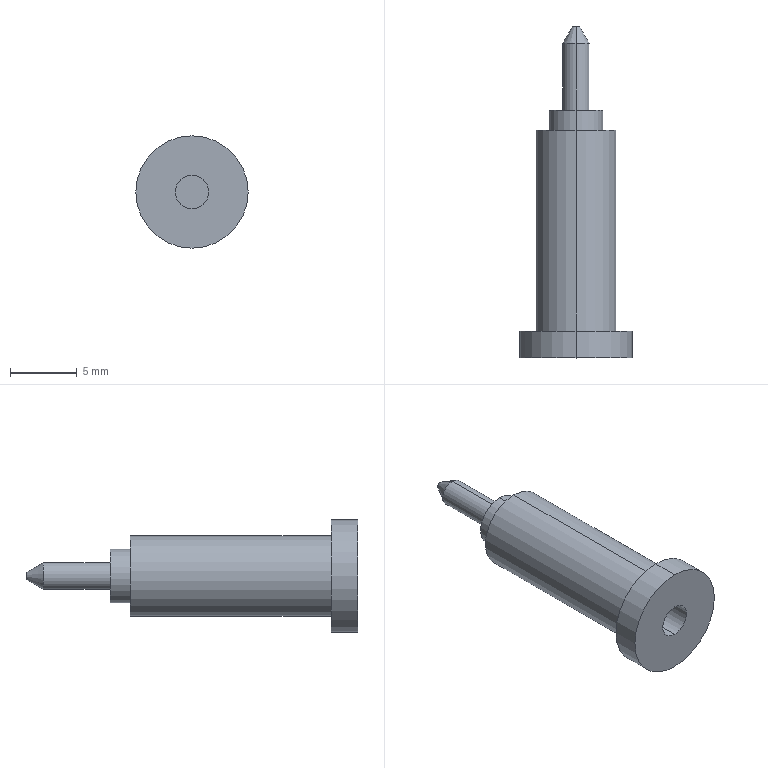Part | SolidWorks | features Revolution 1 | 1 solid | 18 faces | box 8.4 x 24.799 x 8.4 mm | volume 541.841 mm3 | cylinder 10 | plane 6 | cone 2 | commonest cylinder face diameters 2 x2 2.5 x2 4 x2 6 x2 8.4 x2
STEP:
#1=CARTESIAN_POINT('',(0.,6.,1.25));
#2=VERTEX_POINT('',#1);
#3=CARTESIAN_POINT('',(0.,6.,-1.25));
#4=VERTEX_POINT('',#3);
#5=CARTESIAN_POINT('',(0.,6.,0.));
#6=DIRECTION('',(0.,-1.,0.));
#7=DIRECTION('',(0.,0.,-1.));
#8=AXIS2_PLACEMENT_3D('',#5,#6,#7);
#9=CIRCLE('',#8,1.25);
#10=EDGE_CURVE('',#2,#4,#9,.T.);
#11=ORIENTED_EDGE('',*,*,#10,.F.);
#12=CARTESIAN_POINT('',(0.,0.,1.25));
#13=VERTEX_POINT('',#12);
#14=CARTESIAN_POINT('',(0.,0.,1.25));
#15=DIRECTION('',(0.,-1.,0.));
#16=VECTOR('',#15,1000.);
#17=LINE('',#14,#16);
#18=EDGE_CURVE('',#2,#13,#17,.T.);
#19=ORIENTED_EDGE('',*,*,#18,.T.);
#20=CARTESIAN_POINT('',(0.,0.,-1.25));
#21=VERTEX_POINT('',#20);
#22=CARTESIAN_POINT('',(0.,0.,0.));
#23=DIRECTION('',(0.,-1.,0.));
#24=DIRECTION('',(0.,0.,-1.));
#25=AXIS2_PLACEMENT_3D('',#22,#23,#24);
#26=CIRCLE('',#25,1.25);
#27=EDGE_CURVE('',#13,#21,#26,.T.);
#28=ORIENTED_EDGE('',*,*,#27,.T.);
#29=CARTESIAN_POINT('',(0.,0.,-1.25));
#30=DIRECTION('',(0.,-1.,0.));
#31=VECTOR('',#30,1000.);
#32=LINE('',#29,#31);
#33=EDGE_CURVE('',#4,#21,#32,.T.);
#34=ORIENTED_EDGE('',*,*,#33,.F.);
#35=EDGE_LOOP('',(#11,#19,#28,#34));
#36=FACE_OUTER_BOUND('',#35,.T.);
#37=CARTESIAN_POINT('',(0.,0.,0.));
#38=DIRECTION('',(0.,-1.,0.));
#39=DIRECTION('',(0.,0.,-1.));
#40=AXIS2_PLACEMENT_3D('',#37,#38,#39);
#41=CYLINDRICAL_SURFACE('',#40,1.25);
#42=ADVANCED_FACE('',(#36),#41,.F.);
#43=CARTESIAN_POINT('',(0.,24.799,-0.25));
#44=VERTEX_POINT('',#43);
#45=CARTESIAN_POINT('',(0.,24.799,0.25));
#46=VERTEX_POINT('',#45);
#47=CARTESIAN_POINT('',(0.,24.799,0.));
#48=DIRECTION('',(0.,-1.,0.));
#49=DIRECTION('',(0.,0.,-1.));
#50=AXIS2_PLACEMENT_3D('',#47,#48,#49);
#51=CIRCLE('',#50,0.25);
#52=EDGE_CURVE('',#44,#46,#51,.T.);
#53=ORIENTED_EDGE('',*,*,#52,.T.);
#54=CARTESIAN_POINT('',(0.,23.5,1.));
#55=VERTEX_POINT('',#54);
#56=CARTESIAN_POINT('',(0.,24.799,0.25));
#57=DIRECTION('',(0.,-0.866,0.5));
#58=VECTOR('',#57,1000.);
#59=LINE('',#56,#58);
#60=EDGE_CURVE('',#46,#55,#59,.T.);
#61=ORIENTED_EDGE('',*,*,#60,.T.);
#62=CARTESIAN_POINT('',(0.,23.5,-1.));
#63=VERTEX_POINT('',#62);
#64=CARTESIAN_POINT('',(0.,23.5,0.));
#65=DIRECTION('',(0.,-1.,0.));
#66=DIRECTION('',(0.,0.,-1.));
#67=AXIS2_PLACEMENT_3D('',#64,#65,#66);
#68=CIRCLE('',#67,1.);
#69=EDGE_CURVE('',#63,#55,#68,.T.);
#70=ORIENTED_EDGE('',*,*,#69,.F.);
#71=CARTESIAN_POINT('',(0.,24.799,-0.25));
#72=DIRECTION('',(0.,-0.866,-0.5));
#73=VECTOR('',#72,1000.);
#74=LINE('',#71,#73);
#75=EDGE_CURVE('',#44,#63,#74,.T.);
#76=ORIENTED_EDGE('',*,*,#75,.F.);
#77=EDGE_LOOP('',(#53,#61,#70,#76));
#78=FACE_OUTER_BOUND('',#77,.T.);
#79=CARTESIAN_POINT('',(0.,24.799,0.));
#80=DIRECTION('',(0.,-1.,0.));
#81=DIRECTION('',(0.,0.,-1.));
#82=AXIS2_PLACEMENT_3D('',#79,#80,#81);
#83=CONICAL_SURFACE('',#82,0.25,0.5236);
#84=ADVANCED_FACE('',(#78),#83,.T.);
#85=ORIENTED_EDGE('',*,*,#69,.T.);
#86=CARTESIAN_POINT('',(0.,18.5,1.));
#87=VERTEX_POINT('',#86);
#88=CARTESIAN_POINT('',(0.,0.,1.));
#89=DIRECTION('',(0.,-1.,0.));
#90=VECTOR('',#89,1000.);
#91=LINE('',#88,#90);
#92=EDGE_CURVE('',#55,#87,#91,.T.);
#93=ORIENTED_EDGE('',*,*,#92,.T.);
#94=CARTESIAN_POINT('',(0.,18.5,-1.));
#95=VERTEX_POINT('',#94);
#96=CARTESIAN_POINT('',(0.,18.5,0.));
#97=DIRECTION('',(0.,-1.,0.));
#98=DIRECTION('',(0.,0.,-1.));
#99=AXIS2_PLACEMENT_3D('',#96,#97,#98);
#100=CIRCLE('',#99,1.);
#101=EDGE_CURVE('',#95,#87,#100,.T.);
#102=ORIENTED_EDGE('',*,*,#101,.F.);
#103=CARTESIAN_POINT('',(0.,0.,-1.));
#104=DIRECTION('',(0.,-1.,0.));
#105=VECTOR('',#104,1000.);
#106=LINE('',#103,#105);
#107=EDGE_CURVE('',#63,#95,#106,.T.);
#108=ORIENTED_EDGE('',*,*,#107,.F.);
#109=EDGE_LOOP('',(#85,#93,#102,#108));
#110=FACE_OUTER_BOUND('',#109,.T.);
#111=CARTESIAN_POINT('',(0.,0.,0.));
#112=DIRECTION('',(0.,-1.,0.));
#113=DIRECTION('',(0.,0.,-1.));
#114=AXIS2_PLACEMENT_3D('',#111,#112,#113);
#115=CYLINDRICAL_SURFACE('',#114,1.);
#116=ADVANCED_FACE('',(#110),#115,.T.);
#117=CARTESIAN_POINT('',(0.,18.5,-2.));
#118=VERTEX_POINT('',#117);
#119=CARTESIAN_POINT('',(0.,18.5,2.));
#120=VERTEX_POINT('',#119);
#121=CARTESIAN_POINT('',(0.,18.5,0.));
#122=DIRECTION('',(0.,-1.,0.));
#123=DIRECTION('',(0.,0.,-1.));
#124=AXIS2_PLACEMENT_3D('',#121,#122,#123);
#125=CIRCLE('',#124,2.);
#126=EDGE_CURVE('',#118,#120,#125,.T.);
#127=ORIENTED_EDGE('',*,*,#126,.T.);
#128=CARTESIAN_POINT('',(0.,17.,2.));
#129=VERTEX_POINT('',#128);
#130=CARTESIAN_POINT('',(0.,0.,2.));
#131=DIRECTION('',(0.,-1.,0.));
#132=VECTOR('',#131,1000.);
#133=LINE('',#130,#132);
#134=EDGE_CURVE('',#120,#129,#133,.T.);
#135=ORIENTED_EDGE('',*,*,#134,.T.);
#136=CARTESIAN_POINT('',(0.,17.,-2.));
#137=VERTEX_POINT('',#136);
#138=CARTESIAN_POINT('',(0.,17.,0.));
#139=DIRECTION('',(0.,-1.,0.));
#140=DIRECTION('',(0.,0.,-1.));
#141=AXIS2_PLACEMENT_3D('',#138,#139,#140);
#142=CIRCLE('',#141,2.);
#143=EDGE_CURVE('',#137,#129,#142,.T.);
#144=ORIENTED_EDGE('',*,*,#143,.F.);
#145=CARTESIAN_POINT('',(0.,0.,-2.));
#146=DIRECTION('',(0.,-1.,0.));
#147=VECTOR('',#146,1000.);
#148=LINE('',#145,#147);
#149=EDGE_CURVE('',#118,#137,#148,.T.);
#150=ORIENTED_EDGE('',*,*,#149,.F.);
#151=EDGE_LOOP('',(#127,#135,#144,#150));
#152=FACE_OUTER_BOUND('',#151,.T.);
#153=CARTESIAN_POINT('',(0.,0.,0.));
#154=DIRECTION('',(0.,-1.,0.));
#155=DIRECTION('',(0.,0.,-1.));
#156=AXIS2_PLACEMENT_3D('',#153,#154,#155);
#157=CYLINDRICAL_SURFACE('',#156,2.);
#158=ADVANCED_FACE('',(#152),#157,.T.);
#159=CARTESIAN_POINT('',(0.,17.,-3.));
#160=VERTEX_POINT('',#159);
#161=CARTESIAN_POINT('',(0.,17.,3.));
#162=VERTEX_POINT('',#161);
#163=CARTESIAN_POINT('',(0.,17.,0.));
#164=DIRECTION('',(0.,-1.,0.));
#165=DIRECTION('',(0.,0.,-1.));
#166=AXIS2_PLACEMENT_3D('',#163,#164,#165);
#167=CIRCLE('',#166,3.);
#168=EDGE_CURVE('',#160,#162,#167,.T.);
#169=ORIENTED_EDGE('',*,*,#168,.T.);
#170=CARTESIAN_POINT('',(0.,2.,3.));
#171=VERTEX_POINT('',#170);
#172=CARTESIAN_POINT('',(0.,0.,3.));
#173=DIRECTION('',(0.,-1.,0.));
#174=VECTOR('',#173,1000.);
#175=LINE('',#172,#174);
#176=EDGE_CURVE('',#162,#171,#175,.T.);
#177=ORIENTED_EDGE('',*,*,#176,.T.);
#178=CARTESIAN_POINT('',(0.,2.,-3.));
#179=VERTEX_POINT('',#178);
#180=CARTESIAN_POINT('',(0.,2.,0.));
#181=DIRECTION('',(0.,-1.,0.));
#182=DIRECTION('',(0.,0.,-1.));
#183=AXIS2_PLACEMENT_3D('',#180,#181,#182);
#184=CIRCLE('',#183,3.);
#185=EDGE_CURVE('',#179,#171,#184,.T.);
#186=ORIENTED_EDGE('',*,*,#185,.F.);
#187=CARTESIAN_POINT('',(0.,0.,-3.));
#188=DIRECTION('',(0.,-1.,0.));
#189=VECTOR('',#188,1000.);
#190=LINE('',#187,#189);
#191=EDGE_CURVE('',#160,#179,#190,.T.);
#192=ORIENTED_EDGE('',*,*,#191,.F.);
#193=EDGE_LOOP('',(#169,#177,#186,#192));
#194=FACE_OUTER_BOUND('',#193,.T.);
#195=CARTESIAN_POINT('',(0.,0.,0.));
#196=DIRECTION('',(0.,-1.,0.));
#197=DIRECTION('',(0.,0.,-1.));
#198=AXIS2_PLACEMENT_3D('',#195,#196,#197);
#199=CYLINDRICAL_SURFACE('',#198,3.);
#200=ADVANCED_FACE('',(#194),#199,.T.);
#201=CARTESIAN_POINT('',(0.,2.,-4.2));
#202=VERTEX_POINT('',#201);
#203=CARTESIAN_POINT('',(0.,2.,4.2));
#204=VERTEX_POINT('',#203);
#205=CARTESIAN_POINT('',(0.,2.,0.));
#206=DIRECTION('',(0.,-1.,0.));
#207=DIRECTION('',(0.,0.,-1.));
#208=AXIS2_PLACEMENT_3D('',#205,#206,#207);
#209=CIRCLE('',#208,4.2);
#210=EDGE_CURVE('',#202,#204,#209,.T.);
#211=ORIENTED_EDGE('',*,*,#210,.T.);
#212=CARTESIAN_POINT('',(0.,0.,4.2));
#213=VERTEX_POINT('',#212);
#214=CARTESIAN_POINT('',(0.,0.,4.2));
#215=DIRECTION('',(0.,-1.,0.));
#216=VECTOR('',#215,1000.);
#217=LINE('',#214,#216);
#218=EDGE_CURVE('',#204,#213,#217,.T.);
#219=ORIENTED_EDGE('',*,*,#218,.T.);
#220=CARTESIAN_POINT('',(0.,0.,-4.2));
#221=VERTEX_POINT('',#220);
#222=CARTESIAN_POINT('',(0.,0.,0.));
#223=DIRECTION('',(0.,-1.,0.));
#224=DIRECTION('',(0.,0.,-1.));
#225=AXIS2_PLACEMENT_3D('',#222,#223,#224);
#226=CIRCLE('',#225,4.2);
#227=EDGE_CURVE('',#221,#213,#226,.T.);
#228=ORIENTED_EDGE('',*,*,#227,.F.);
#229=CARTESIAN_POINT('',(0.,0.,-4.2));
#230=DIRECTION('',(0.,-1.,0.));
#231=VECTOR('',#230,1000.);
#232=LINE('',#229,#231);
#233=EDGE_CURVE('',#202,#221,#232,.T.);
#234=ORIENTED_EDGE('',*,*,#233,.F.);
#235=EDGE_LOOP('',(#211,#219,#228,#234));
#236=FACE_OUTER_BOUND('',#235,.T.);
#237=CARTESIAN_POINT('',(0.,0.,0.));
#238=DIRECTION('',(0.,-1.,0.));
#239=DIRECTION('',(0.,0.,-1.));
#240=AXIS2_PLACEMENT_3D('',#237,#238,#239);
#241=CYLINDRICAL_SURFACE('',#240,4.2);
#242=ADVANCED_FACE('',(#236),#241,.T.);
#243=ORIENTED_EDGE('',*,*,#218,.F.);
#244=CARTESIAN_POINT('',(0.,2.,0.));
#245=DIRECTION('',(0.,-1.,0.));
#246=DIRECTION('',(0.,0.,-1.));
#247=AXIS2_PLACEMENT_3D('',#244,#245,#246);
#248=CIRCLE('',#247,4.2);
#249=EDGE_CURVE('',#204,#202,#248,.T.);
#250=ORIENTED_EDGE('',*,*,#249,.T.);
#251=ORIENTED_EDGE('',*,*,#233,.T.);
#252=CARTESIAN_POINT('',(0.,0.,0.));
#253=DIRECTION('',(0.,-1.,0.));
#254=DIRECTION('',(0.,0.,-1.));
#255=AXIS2_PLACEMENT_3D('',#252,#253,#254);
#256=CIRCLE('',#255,4.2);
#257=EDGE_CURVE('',#213,#221,#256,.T.);
#258=ORIENTED_EDGE('',*,*,#257,.F.);
#259=EDGE_LOOP('',(#243,#250,#251,#258));
#260=FACE_OUTER_BOUND('',#259,.T.);
#261=CARTESIAN_POINT('',(0.,0.,0.));
#262=DIRECTION('',(0.,-1.,0.));
#263=DIRECTION('',(0.,0.,-1.));
#264=AXIS2_PLACEMENT_3D('',#261,#262,#263);
#265=CYLINDRICAL_SURFACE('',#264,4.2);
#266=ADVANCED_FACE('',(#260),#265,.T.);
#267=ORIENTED_EDGE('',*,*,#210,.F.);
#268=ORIENTED_EDGE('',*,*,#249,.F.);
#269=EDGE_LOOP('',(#267,#268));
#270=FACE_OUTER_BOUND('',#269,.T.);
#271=ORIENTED_EDGE('',*,*,#185,.T.);
#272=CARTESIAN_POINT('',(0.,2.,0.));
#273=DIRECTION('',(0.,-1.,0.));
#274=DIRECTION('',(0.,0.,-1.));
#275=AXIS2_PLACEMENT_3D('',#272,#273,#274);
#276=CIRCLE('',#275,3.);
#277=EDGE_CURVE('',#171,#179,#276,.T.);
#278=ORIENTED_EDGE('',*,*,#277,.T.);
#279=EDGE_LOOP('',(#271,#278));
#280=FACE_BOUND('',#279,.T.);
#281=CARTESIAN_POINT('',(-4.2,2.,0.));
#282=DIRECTION('',(0.,-1.,0.));
#283=DIRECTION('',(0.,0.,-1.));
#284=AXIS2_PLACEMENT_3D('',#281,#282,#283);
#285=PLANE('',#284);
#286=ADVANCED_FACE('',(#270,#280),#285,.F.);
#287=ORIENTED_EDGE('',*,*,#176,.F.);
#288=CARTESIAN_POINT('',(0.,17.,0.));
#289=DIRECTION('',(0.,-1.,0.));
#290=DIRECTION('',(0.,0.,-1.));
#291=AXIS2_PLACEMENT_3D('',#288,#289,#290);
#292=CIRCLE('',#291,3.);
#293=EDGE_CURVE('',#162,#160,#292,.T.);
#294=ORIENTED_EDGE('',*,*,#293,.T.);
#295=ORIENTED_EDGE('',*,*,#191,.T.);
#296=ORIENTED_EDGE('',*,*,#277,.F.);
#297=EDGE_LOOP('',(#287,#294,#295,#296));
#298=FACE_OUTER_BOUND('',#297,.T.);
#299=CARTESIAN_POINT('',(0.,0.,0.));
#300=DIRECTION('',(0.,-1.,0.));
#301=DIRECTION('',(0.,0.,-1.));
#302=AXIS2_PLACEMENT_3D('',#299,#300,#301);
#303=CYLINDRICAL_SURFACE('',#302,3.);
#304=ADVANCED_FACE('',(#298),#303,.T.);
#305=ORIENTED_EDGE('',*,*,#168,.F.);
#306=ORIENTED_EDGE('',*,*,#293,.F.);
#307=EDGE_LOOP('',(#305,#306));
#308=FACE_OUTER_BOUND('',#307,.T.);
#309=ORIENTED_EDGE('',*,*,#143,.T.);
#310=CARTESIAN_POINT('',(0.,17.,0.));
#311=DIRECTION('',(0.,-1.,0.));
#312=DIRECTION('',(0.,0.,-1.));
#313=AXIS2_PLACEMENT_3D('',#310,#311,#312);
#314=CIRCLE('',#313,2.);
#315=EDGE_CURVE('',#129,#137,#314,.T.);
#316=ORIENTED_EDGE('',*,*,#315,.T.);
#317=EDGE_LOOP('',(#309,#316));
#318=FACE_BOUND('',#317,.T.);
#319=CARTESIAN_POINT('',(-3.,17.,0.));
#320=DIRECTION('',(0.,-1.,0.));
#321=DIRECTION('',(0.,0.,-1.));
#322=AXIS2_PLACEMENT_3D('',#319,#320,#321);
#323=PLANE('',#322);
#324=ADVANCED_FACE('',(#308,#318),#323,.F.);
#325=ORIENTED_EDGE('',*,*,#134,.F.);
#326=CARTESIAN_POINT('',(0.,18.5,0.));
#327=DIRECTION('',(0.,-1.,0.));
#328=DIRECTION('',(0.,0.,-1.));
#329=AXIS2_PLACEMENT_3D('',#326,#327,#328);
#330=CIRCLE('',#329,2.);
#331=EDGE_CURVE('',#120,#118,#330,.T.);
#332=ORIENTED_EDGE('',*,*,#331,.T.);
#333=ORIENTED_EDGE('',*,*,#149,.T.);
#334=ORIENTED_EDGE('',*,*,#315,.F.);
#335=EDGE_LOOP('',(#325,#332,#333,#334));
#336=FACE_OUTER_BOUND('',#335,.T.);
#337=CARTESIAN_POINT('',(0.,0.,0.));
#338=DIRECTION('',(0.,-1.,0.));
#339=DIRECTION('',(0.,0.,-1.));
#340=AXIS2_PLACEMENT_3D('',#337,#338,#339);
#341=CYLINDRICAL_SURFACE('',#340,2.);
#342=ADVANCED_FACE('',(#336),#341,.T.);
#343=ORIENTED_EDGE('',*,*,#126,.F.);
#344=ORIENTED_EDGE('',*,*,#331,.F.);
#345=EDGE_LOOP('',(#343,#344));
#346=FACE_OUTER_BOUND('',#345,.T.);
#347=ORIENTED_EDGE('',*,*,#101,.T.);
#348=CARTESIAN_POINT('',(0.,18.5,0.));
#349=DIRECTION('',(0.,-1.,0.));
#350=DIRECTION('',(0.,0.,-1.));
#351=AXIS2_PLACEMENT_3D('',#348,#349,#350);
#352=CIRCLE('',#351,1.);
#353=EDGE_CURVE('',#87,#95,#352,.T.);
#354=ORIENTED_EDGE('',*,*,#353,.T.);
#355=EDGE_LOOP('',(#347,#354));
#356=FACE_BOUND('',#355,.T.);
#357=CARTESIAN_POINT('',(-2.,18.5,0.));
#358=DIRECTION('',(0.,-1.,0.));
#359=DIRECTION('',(0.,0.,-1.));
#360=AXIS2_PLACEMENT_3D('',#357,#358,#359);
#361=PLANE('',#360);
#362=ADVANCED_FACE('',(#346,#356),#361,.F.);
#363=ORIENTED_EDGE('',*,*,#92,.F.);
#364=CARTESIAN_POINT('',(0.,23.5,0.));
#365=DIRECTION('',(0.,-1.,0.));
#366=DIRECTION('',(0.,0.,-1.));
#367=AXIS2_PLACEMENT_3D('',#364,#365,#366);
#368=CIRCLE('',#367,1.);
#369=EDGE_CURVE('',#55,#63,#368,.T.);
#370=ORIENTED_EDGE('',*,*,#369,.T.);
#371=ORIENTED_EDGE('',*,*,#107,.T.);
#372=ORIENTED_EDGE('',*,*,#353,.F.);
#373=EDGE_LOOP('',(#363,#370,#371,#372));
#374=FACE_OUTER_BOUND('',#373,.T.);
#375=CARTESIAN_POINT('',(0.,0.,0.));
#376=DIRECTION('',(0.,-1.,0.));
#377=DIRECTION('',(0.,0.,-1.));
#378=AXIS2_PLACEMENT_3D('',#375,#376,#377);
#379=CYLINDRICAL_SURFACE('',#378,1.);
#380=ADVANCED_FACE('',(#374),#379,.T.);
#381=ORIENTED_EDGE('',*,*,#60,.F.);
#382=CARTESIAN_POINT('',(0.,24.799,0.));
#383=DIRECTION('',(0.,-1.,0.));
#384=DIRECTION('',(0.,0.,-1.));
#385=AXIS2_PLACEMENT_3D('',#382,#383,#384);
#386=CIRCLE('',#385,0.25);
#387=EDGE_CURVE('',#46,#44,#386,.T.);
#388=ORIENTED_EDGE('',*,*,#387,.T.);
#389=ORIENTED_EDGE('',*,*,#75,.T.);
#390=ORIENTED_EDGE('',*,*,#369,.F.);
#391=EDGE_LOOP('',(#381,#388,#389,#390));
#392=FACE_OUTER_BOUND('',#391,.T.);
#393=CARTESIAN_POINT('',(0.,24.799,0.));
#394=DIRECTION('',(0.,-1.,0.));
#395=DIRECTION('',(0.,0.,-1.));
#396=AXIS2_PLACEMENT_3D('',#393,#394,#395);
#397=CONICAL_SURFACE('',#396,0.25,0.5236);
#398=ADVANCED_FACE('',(#392),#397,.T.);
#399=ORIENTED_EDGE('',*,*,#52,.F.);
#400=ORIENTED_EDGE('',*,*,#387,.F.);
#401=EDGE_LOOP('',(#399,#400));
#402=FACE_OUTER_BOUND('',#401,.T.);
#403=CARTESIAN_POINT('',(-0.25,24.799,0.));
#404=DIRECTION('',(0.,-1.,0.));
#405=DIRECTION('',(0.,0.,-1.));
#406=AXIS2_PLACEMENT_3D('',#403,#404,#405);
#407=PLANE('',#406);
#408=ADVANCED_FACE('',(#402),#407,.F.);
#409=CARTESIAN_POINT('',(0.,6.,0.));
#410=DIRECTION('',(0.,-1.,0.));
#411=DIRECTION('',(0.,0.,-1.));
#412=AXIS2_PLACEMENT_3D('',#409,#410,#411);
#413=CIRCLE('',#412,1.25);
#414=EDGE_CURVE('',#4,#2,#413,.T.);
#415=ORIENTED_EDGE('',*,*,#414,.T.);
#416=ORIENTED_EDGE('',*,*,#10,.T.);
#417=EDGE_LOOP('',(#415,#416));
#418=FACE_OUTER_BOUND('',#417,.T.);
#419=CARTESIAN_POINT('',(-1.25,6.,0.));
#420=DIRECTION('',(0.,1.,0.));
#421=DIRECTION('',(0.,0.,1.));
#422=AXIS2_PLACEMENT_3D('',#419,#420,#421);
#423=PLANE('',#422);
#424=ADVANCED_FACE('',(#418),#423,.F.);
#425=ORIENTED_EDGE('',*,*,#18,.F.);
#426=ORIENTED_EDGE('',*,*,#414,.F.);
#427=ORIENTED_EDGE('',*,*,#33,.T.);
#428=CARTESIAN_POINT('',(0.,0.,0.));
#429=DIRECTION('',(0.,-1.,0.));
#430=DIRECTION('',(0.,0.,-1.));
#431=AXIS2_PLACEMENT_3D('',#428,#429,#430);
#432=CIRCLE('',#431,1.25);
#433=EDGE_CURVE('',#21,#13,#432,.T.);
#434=ORIENTED_EDGE('',*,*,#433,.T.);
#435=EDGE_LOOP('',(#425,#426,#427,#434));
#436=FACE_OUTER_BOUND('',#435,.T.);
#437=CARTESIAN_POINT('',(0.,0.,0.));
#438=DIRECTION('',(0.,-1.,0.));
#439=DIRECTION('',(0.,0.,-1.));
#440=AXIS2_PLACEMENT_3D('',#437,#438,#439);
#441=CYLINDRICAL_SURFACE('',#440,1.25);
#442=ADVANCED_FACE('',(#436),#441,.F.);
#443=ORIENTED_EDGE('',*,*,#433,.F.);
#444=ORIENTED_EDGE('',*,*,#27,.F.);
#445=EDGE_LOOP('',(#443,#444));
#446=FACE_BOUND('',#445,.T.);
#447=ORIENTED_EDGE('',*,*,#227,.T.);
#448=ORIENTED_EDGE('',*,*,#257,.T.);
#449=EDGE_LOOP('',(#447,#448));
#450=FACE_OUTER_BOUND('',#449,.T.);
#451=CARTESIAN_POINT('',(-1.25,0.,0.));
#452=DIRECTION('',(0.,1.,0.));
#453=DIRECTION('',(0.,0.,1.));
#454=AXIS2_PLACEMENT_3D('',#451,#452,#453);
#455=PLANE('',#454);
#456=ADVANCED_FACE('',(#446,#450),#455,.F.);
#457=CLOSED_SHELL('',(#42,#84,#116,#158,#200,#242,#266,#286,#304,#324,#342,#362,#380,#398,#408,#424,#442,#456));
#458=MANIFOLD_SOLID_BREP('',#457);
#459=CARTESIAN_POINT('',(0.,0.,0.));
#460=DIRECTION('',(0.,0.,1.));
#461=DIRECTION('',(1.,0.,0.));
#462=AXIS2_PLACEMENT_3D('',#459,#460,#461);
#463=(LENGTH_UNIT()NAMED_UNIT(*)SI_UNIT(.MILLI.,.METRE.));
#464=UNCERTAINTY_MEASURE_WITH_UNIT(LENGTH_MEASURE(0.00001),#463,'','');
#465=(NAMED_UNIT(*)PLANE_ANGLE_UNIT()SI_UNIT($,.RADIAN.));
#466=(NAMED_UNIT(*)SI_UNIT($,.STERADIAN.)SOLID_ANGLE_UNIT());
#467=(GEOMETRIC_REPRESENTATION_CONTEXT(3)GLOBAL_UNCERTAINTY_ASSIGNED_CONTEXT((#464))GLOBAL_UNIT_ASSIGNED_CONTEXT((#463,#465,#466))REPRESENTATION_CONTEXT('',''));
#468=ADVANCED_BREP_SHAPE_REPRESENTATION('',(#458,#462),#467);